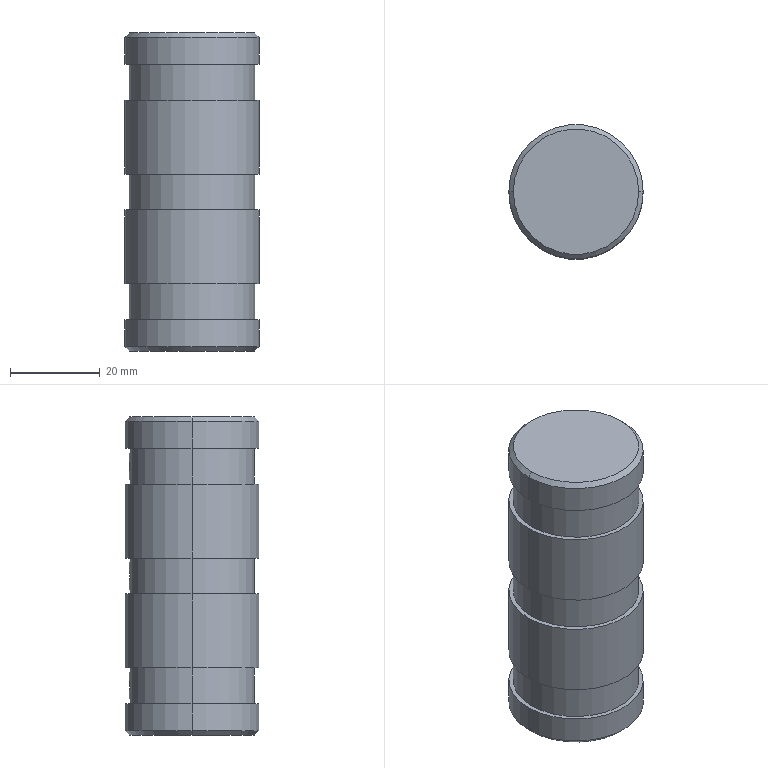Part | SolidWorks | features HoleWzd 3, 3DProfileFeature 2, Chamfer 1, Extrusion 1, ICE 1, RevCut 1 | 1 solid | 58 faces | box 30 x 30 x 71 mm | volume 47169 mm3 | cylinder 36 | cone 14 | plane 8 | commonest cylinder face diameters 3 x20 30 x8 28 x6 3.3 x2